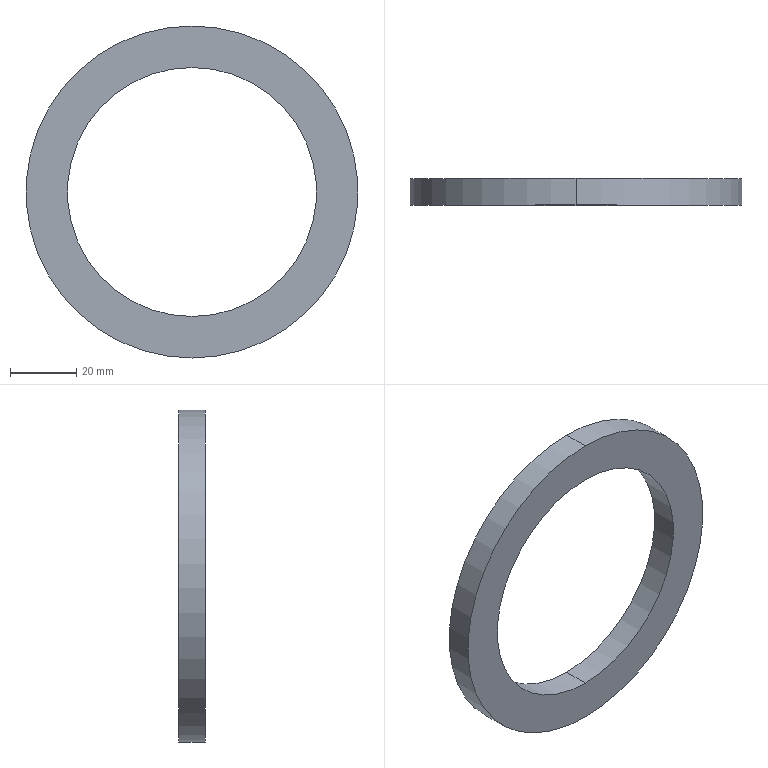Part | NX | features BREP 1 | 1 solid | 6 faces | box 100 x 8 x 100 mm | volume 27489 mm3 | cylinder 4 | plane 2 | commonest cylinder face diameters 75 x2 100 x2
STEP:
#1=CARTESIAN_POINT('',(0.,4.,-37.5));
#2=VERTEX_POINT('',#1);
#3=CARTESIAN_POINT('',(0.,4.,37.5));
#4=VERTEX_POINT('',#3);
#5=CARTESIAN_POINT('',(0.,4.,0.));
#6=DIRECTION('',(0.,1.,0.));
#7=DIRECTION('',(0.,0.,1.));
#8=AXIS2_PLACEMENT_3D('',#5,#6,#7);
#9=CIRCLE('',#8,37.5);
#10=EDGE_CURVE('',#2,#4,#9,.T.);
#11=ORIENTED_EDGE('',*,*,#10,.T.);
#12=CARTESIAN_POINT('',(0.,-4.,37.5));
#13=VERTEX_POINT('',#12);
#14=CARTESIAN_POINT('',(0.,4.,37.5));
#15=DIRECTION('',(0.,-1.,0.));
#16=VECTOR('',#15,1000.);
#17=LINE('',#14,#16);
#18=EDGE_CURVE('',#13,#4,#17,.F.);
#19=ORIENTED_EDGE('',*,*,#18,.F.);
#20=CARTESIAN_POINT('',(0.,-4.,-37.5));
#21=VERTEX_POINT('',#20);
#22=CARTESIAN_POINT('',(0.,-4.,0.));
#23=DIRECTION('',(0.,1.,0.));
#24=DIRECTION('',(0.,0.,1.));
#25=AXIS2_PLACEMENT_3D('',#22,#23,#24);
#26=CIRCLE('',#25,37.5);
#27=EDGE_CURVE('',#21,#13,#26,.T.);
#28=ORIENTED_EDGE('',*,*,#27,.F.);
#29=CARTESIAN_POINT('',(0.,4.,-37.5));
#30=DIRECTION('',(0.,-1.,0.));
#31=VECTOR('',#30,1000.);
#32=LINE('',#29,#31);
#33=EDGE_CURVE('',#21,#2,#32,.F.);
#34=ORIENTED_EDGE('',*,*,#33,.T.);
#35=EDGE_LOOP('',(#11,#19,#28,#34));
#36=FACE_BOUND('',#35,.T.);
#37=CARTESIAN_POINT('',(0.,4.,0.));
#38=DIRECTION('',(0.,-1.,0.));
#39=DIRECTION('',(0.,0.,1.));
#40=AXIS2_PLACEMENT_3D('',#37,#38,#39);
#41=CYLINDRICAL_SURFACE('',#40,37.5);
#42=ADVANCED_FACE('',(#36),#41,.F.);
#43=CARTESIAN_POINT('',(0.,4.,50.));
#44=VERTEX_POINT('',#43);
#45=CARTESIAN_POINT('',(0.,4.,-50.));
#46=VERTEX_POINT('',#45);
#47=CARTESIAN_POINT('',(0.,4.,0.));
#48=DIRECTION('',(0.,1.,0.));
#49=DIRECTION('',(0.,0.,1.));
#50=AXIS2_PLACEMENT_3D('',#47,#48,#49);
#51=CIRCLE('',#50,50.);
#52=EDGE_CURVE('',#44,#46,#51,.T.);
#53=ORIENTED_EDGE('',*,*,#52,.F.);
#54=CARTESIAN_POINT('',(0.,-4.,50.));
#55=VERTEX_POINT('',#54);
#56=CARTESIAN_POINT('',(0.,4.,50.));
#57=DIRECTION('',(0.,-1.,0.));
#58=VECTOR('',#57,1000.);
#59=LINE('',#56,#58);
#60=EDGE_CURVE('',#55,#44,#59,.F.);
#61=ORIENTED_EDGE('',*,*,#60,.F.);
#62=CARTESIAN_POINT('',(0.,-4.,-50.));
#63=VERTEX_POINT('',#62);
#64=CARTESIAN_POINT('',(0.,-4.,0.));
#65=DIRECTION('',(0.,1.,0.));
#66=DIRECTION('',(0.,0.,1.));
#67=AXIS2_PLACEMENT_3D('',#64,#65,#66);
#68=CIRCLE('',#67,50.);
#69=EDGE_CURVE('',#55,#63,#68,.T.);
#70=ORIENTED_EDGE('',*,*,#69,.T.);
#71=CARTESIAN_POINT('',(0.,4.,-50.));
#72=DIRECTION('',(0.,-1.,0.));
#73=VECTOR('',#72,1000.);
#74=LINE('',#71,#73);
#75=EDGE_CURVE('',#63,#46,#74,.F.);
#76=ORIENTED_EDGE('',*,*,#75,.T.);
#77=EDGE_LOOP('',(#53,#61,#70,#76));
#78=FACE_BOUND('',#77,.T.);
#79=CARTESIAN_POINT('',(0.,4.,0.));
#80=DIRECTION('',(0.,-1.,0.));
#81=DIRECTION('',(0.,0.,1.));
#82=AXIS2_PLACEMENT_3D('',#79,#80,#81);
#83=CYLINDRICAL_SURFACE('',#82,50.);
#84=ADVANCED_FACE('',(#78),#83,.T.);
#85=CARTESIAN_POINT('',(0.,4.,0.));
#86=DIRECTION('',(0.,1.,0.));
#87=DIRECTION('',(0.,0.,1.));
#88=AXIS2_PLACEMENT_3D('',#85,#86,#87);
#89=CIRCLE('',#88,50.);
#90=EDGE_CURVE('',#46,#44,#89,.T.);
#91=ORIENTED_EDGE('',*,*,#90,.T.);
#92=ORIENTED_EDGE('',*,*,#52,.T.);
#93=EDGE_LOOP('',(#91,#92));
#94=FACE_BOUND('',#93,.T.);
#95=ORIENTED_EDGE('',*,*,#10,.F.);
#96=CARTESIAN_POINT('',(0.,4.,0.));
#97=DIRECTION('',(0.,1.,0.));
#98=DIRECTION('',(0.,0.,1.));
#99=AXIS2_PLACEMENT_3D('',#96,#97,#98);
#100=CIRCLE('',#99,37.5);
#101=EDGE_CURVE('',#4,#2,#100,.T.);
#102=ORIENTED_EDGE('',*,*,#101,.F.);
#103=EDGE_LOOP('',(#95,#102));
#104=FACE_BOUND('',#103,.T.);
#105=CARTESIAN_POINT('',(0.,4.,0.));
#106=DIRECTION('',(0.,1.,0.));
#107=DIRECTION('',(0.,0.,-1.));
#108=AXIS2_PLACEMENT_3D('',#105,#106,#107);
#109=PLANE('',#108);
#110=ADVANCED_FACE('',(#94,#104),#109,.T.);
#111=CARTESIAN_POINT('',(0.,-4.,0.));
#112=DIRECTION('',(0.,1.,0.));
#113=DIRECTION('',(0.,0.,1.));
#114=AXIS2_PLACEMENT_3D('',#111,#112,#113);
#115=CIRCLE('',#114,50.);
#116=EDGE_CURVE('',#63,#55,#115,.T.);
#117=ORIENTED_EDGE('',*,*,#116,.F.);
#118=ORIENTED_EDGE('',*,*,#69,.F.);
#119=EDGE_LOOP('',(#117,#118));
#120=FACE_BOUND('',#119,.T.);
#121=ORIENTED_EDGE('',*,*,#27,.T.);
#122=CARTESIAN_POINT('',(0.,-4.,0.));
#123=DIRECTION('',(0.,1.,0.));
#124=DIRECTION('',(0.,0.,1.));
#125=AXIS2_PLACEMENT_3D('',#122,#123,#124);
#126=CIRCLE('',#125,37.5);
#127=EDGE_CURVE('',#13,#21,#126,.T.);
#128=ORIENTED_EDGE('',*,*,#127,.T.);
#129=EDGE_LOOP('',(#121,#128));
#130=FACE_BOUND('',#129,.T.);
#131=CARTESIAN_POINT('',(0.,-4.,0.));
#132=DIRECTION('',(0.,1.,0.));
#133=DIRECTION('',(0.,0.,-1.));
#134=AXIS2_PLACEMENT_3D('',#131,#132,#133);
#135=PLANE('',#134);
#136=ADVANCED_FACE('',(#120,#130),#135,.F.);
#137=ORIENTED_EDGE('',*,*,#60,.T.);
#138=ORIENTED_EDGE('',*,*,#90,.F.);
#139=ORIENTED_EDGE('',*,*,#75,.F.);
#140=ORIENTED_EDGE('',*,*,#116,.T.);
#141=EDGE_LOOP('',(#137,#138,#139,#140));
#142=FACE_BOUND('',#141,.T.);
#143=CARTESIAN_POINT('',(0.,4.,0.));
#144=DIRECTION('',(0.,-1.,0.));
#145=DIRECTION('',(0.,0.,1.));
#146=AXIS2_PLACEMENT_3D('',#143,#144,#145);
#147=CYLINDRICAL_SURFACE('',#146,50.);
#148=ADVANCED_FACE('',(#142),#147,.T.);
#149=ORIENTED_EDGE('',*,*,#18,.T.);
#150=ORIENTED_EDGE('',*,*,#101,.T.);
#151=ORIENTED_EDGE('',*,*,#33,.F.);
#152=ORIENTED_EDGE('',*,*,#127,.F.);
#153=EDGE_LOOP('',(#149,#150,#151,#152));
#154=FACE_BOUND('',#153,.T.);
#155=CARTESIAN_POINT('',(0.,4.,0.));
#156=DIRECTION('',(0.,-1.,0.));
#157=DIRECTION('',(0.,0.,1.));
#158=AXIS2_PLACEMENT_3D('',#155,#156,#157);
#159=CYLINDRICAL_SURFACE('',#158,37.5);
#160=ADVANCED_FACE('',(#154),#159,.F.);
#161=CLOSED_SHELL('',(#42,#84,#110,#136,#148,#160));
#162=MANIFOLD_SOLID_BREP('',#161);
#163=(LENGTH_UNIT()NAMED_UNIT(*)SI_UNIT(.MILLI.,.METRE.));
#164=UNCERTAINTY_MEASURE_WITH_UNIT(LENGTH_MEASURE(0.00001),#163,'','');
#165=(NAMED_UNIT(*)PLANE_ANGLE_UNIT()SI_UNIT($,.RADIAN.));
#166=(NAMED_UNIT(*)SI_UNIT($,.STERADIAN.)SOLID_ANGLE_UNIT());
#167=(GEOMETRIC_REPRESENTATION_CONTEXT(3)GLOBAL_UNCERTAINTY_ASSIGNED_CONTEXT((#164))GLOBAL_UNIT_ASSIGNED_CONTEXT((#163,#165,#166))REPRESENTATION_CONTEXT('',''));
#168=ADVANCED_BREP_SHAPE_REPRESENTATION('',(#162),#167);